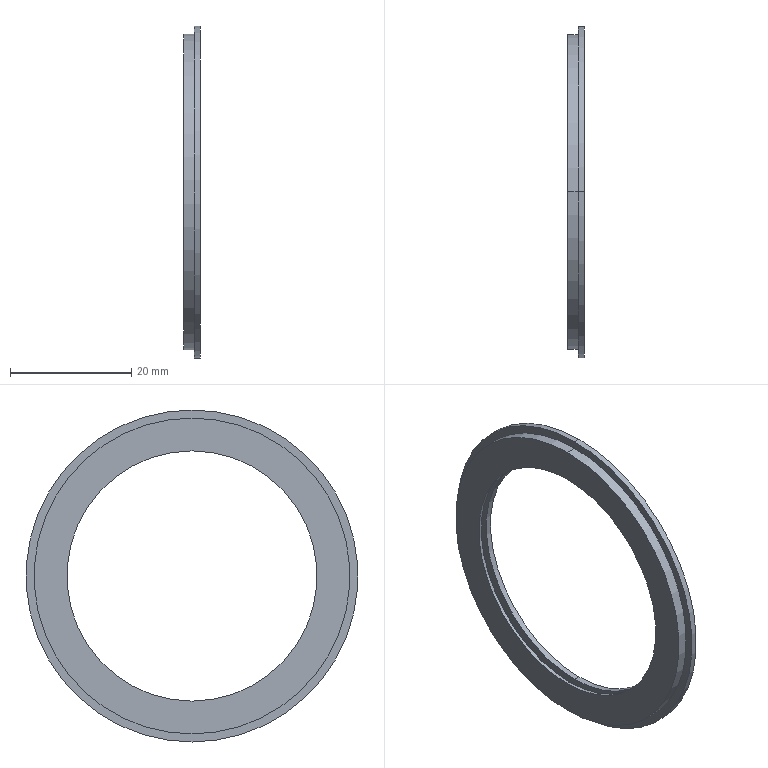Part | SolidWorks | features BaseBody 1 | 1 solid | 15 faces | box 2.7 x 54.668 x 54.668 mm | volume 1535 mm3 | cylinder 10 | plane 5 | commonest cylinder face diameters 41.2 x4 51 x2 52 x2 54.668 x2
STEP:
#1=CARTESIAN_POINT('',(-8.6,63.,15.566));
#2=VERTEX_POINT('',#1);
#3=CARTESIAN_POINT('',(-8.6,63.,70.234));
#4=VERTEX_POINT('',#3);
#5=CARTESIAN_POINT('',(-8.6,63.,42.9));
#6=DIRECTION('',(1.,0.,0.));
#7=DIRECTION('',(0.,0.,-1.));
#8=AXIS2_PLACEMENT_3D('',#5,#6,#7);
#9=CIRCLE('',#8,27.334);
#10=EDGE_CURVE('',#2,#4,#9,.T.);
#11=ORIENTED_EDGE('',*,*,#10,.T.);
#12=CARTESIAN_POINT('',(-7.6,63.,70.234));
#13=VERTEX_POINT('',#12);
#14=CARTESIAN_POINT('',(-8.1,63.,70.234));
#15=DIRECTION('',(1.,0.,0.));
#16=VECTOR('',#15,1000.);
#17=LINE('',#14,#16);
#18=EDGE_CURVE('',#4,#13,#17,.T.);
#19=ORIENTED_EDGE('',*,*,#18,.T.);
#20=CARTESIAN_POINT('',(-7.6,63.,15.566));
#21=VERTEX_POINT('',#20);
#22=CARTESIAN_POINT('',(-7.6,63.,42.9));
#23=DIRECTION('',(1.,0.,0.));
#24=DIRECTION('',(0.,0.,-1.));
#25=AXIS2_PLACEMENT_3D('',#22,#23,#24);
#26=CIRCLE('',#25,27.334);
#27=EDGE_CURVE('',#21,#13,#26,.T.);
#28=ORIENTED_EDGE('',*,*,#27,.F.);
#29=CARTESIAN_POINT('',(-8.1,63.,15.566));
#30=DIRECTION('',(1.,0.,0.));
#31=VECTOR('',#30,1000.);
#32=LINE('',#29,#31);
#33=EDGE_CURVE('',#2,#21,#32,.T.);
#34=ORIENTED_EDGE('',*,*,#33,.F.);
#35=EDGE_LOOP('',(#11,#19,#28,#34));
#36=FACE_OUTER_BOUND('',#35,.T.);
#37=CARTESIAN_POINT('',(-8.1,63.,42.9));
#38=DIRECTION('',(1.,0.,0.));
#39=DIRECTION('',(0.,0.,-1.));
#40=AXIS2_PLACEMENT_3D('',#37,#38,#39);
#41=CYLINDRICAL_SURFACE('',#40,27.334);
#42=ADVANCED_FACE('',(#36),#41,.T.);
#43=CARTESIAN_POINT('',(-8.6,63.,22.3));
#44=VERTEX_POINT('',#43);
#45=CARTESIAN_POINT('',(-8.6,63.,63.5));
#46=VERTEX_POINT('',#45);
#47=CARTESIAN_POINT('',(-8.6,63.,42.9));
#48=DIRECTION('',(-1.,0.,0.));
#49=DIRECTION('',(0.,0.,-1.));
#50=AXIS2_PLACEMENT_3D('',#47,#48,#49);
#51=CIRCLE('',#50,20.6);
#52=EDGE_CURVE('',#44,#46,#51,.T.);
#53=ORIENTED_EDGE('',*,*,#52,.T.);
#54=CARTESIAN_POINT('',(-7.6,63.,63.5));
#55=VERTEX_POINT('',#54);
#56=CARTESIAN_POINT('',(-8.6,63.,63.5));
#57=DIRECTION('',(1.,0.,0.));
#58=VECTOR('',#57,1000.);
#59=LINE('',#56,#58);
#60=EDGE_CURVE('',#46,#55,#59,.T.);
#61=ORIENTED_EDGE('',*,*,#60,.T.);
#62=CARTESIAN_POINT('',(-7.6,63.,22.3));
#63=VERTEX_POINT('',#62);
#64=CARTESIAN_POINT('',(-7.6,63.,42.9));
#65=DIRECTION('',(-1.,0.,0.));
#66=DIRECTION('',(0.,0.,-1.));
#67=AXIS2_PLACEMENT_3D('',#64,#65,#66);
#68=CIRCLE('',#67,20.6);
#69=EDGE_CURVE('',#63,#55,#68,.T.);
#70=ORIENTED_EDGE('',*,*,#69,.F.);
#71=CARTESIAN_POINT('',(-8.6,63.,22.3));
#72=DIRECTION('',(1.,0.,0.));
#73=VECTOR('',#72,1000.);
#74=LINE('',#71,#73);
#75=EDGE_CURVE('',#44,#63,#74,.T.);
#76=ORIENTED_EDGE('',*,*,#75,.F.);
#77=EDGE_LOOP('',(#53,#61,#70,#76));
#78=FACE_OUTER_BOUND('',#77,.T.);
#79=CARTESIAN_POINT('',(-8.6,63.,42.9));
#80=DIRECTION('',(1.,0.,0.));
#81=DIRECTION('',(0.,0.,-1.));
#82=AXIS2_PLACEMENT_3D('',#79,#80,#81);
#83=CYLINDRICAL_SURFACE('',#82,20.6);
#84=ADVANCED_FACE('',(#78),#83,.F.);
#85=CARTESIAN_POINT('',(-10.3,63.,16.9));
#86=VERTEX_POINT('',#85);
#87=CARTESIAN_POINT('',(-10.3,63.,68.9));
#88=VERTEX_POINT('',#87);
#89=CARTESIAN_POINT('',(-10.3,63.,42.9));
#90=DIRECTION('',(1.,0.,0.));
#91=DIRECTION('',(0.,0.,-1.));
#92=AXIS2_PLACEMENT_3D('',#89,#90,#91);
#93=CIRCLE('',#92,26.);
#94=EDGE_CURVE('',#86,#88,#93,.T.);
#95=ORIENTED_EDGE('',*,*,#94,.T.);
#96=CARTESIAN_POINT('',(-8.6,63.,68.9));
#97=VERTEX_POINT('',#96);
#98=CARTESIAN_POINT('',(-9.45,63.,68.9));
#99=DIRECTION('',(1.,0.,0.));
#100=VECTOR('',#99,1000.);
#101=LINE('',#98,#100);
#102=EDGE_CURVE('',#88,#97,#101,.T.);
#103=ORIENTED_EDGE('',*,*,#102,.T.);
#104=CARTESIAN_POINT('',(-8.6,63.,16.9));
#105=VERTEX_POINT('',#104);
#106=CARTESIAN_POINT('',(-8.6,63.,42.9));
#107=DIRECTION('',(1.,0.,0.));
#108=DIRECTION('',(0.,0.,-1.));
#109=AXIS2_PLACEMENT_3D('',#106,#107,#108);
#110=CIRCLE('',#109,26.);
#111=EDGE_CURVE('',#105,#97,#110,.T.);
#112=ORIENTED_EDGE('',*,*,#111,.F.);
#113=CARTESIAN_POINT('',(-9.45,63.,16.9));
#114=DIRECTION('',(1.,0.,0.));
#115=VECTOR('',#114,1000.);
#116=LINE('',#113,#115);
#117=EDGE_CURVE('',#86,#105,#116,.T.);
#118=ORIENTED_EDGE('',*,*,#117,.F.);
#119=EDGE_LOOP('',(#95,#103,#112,#118));
#120=FACE_OUTER_BOUND('',#119,.T.);
#121=CARTESIAN_POINT('',(-9.45,63.,42.9));
#122=DIRECTION('',(1.,0.,0.));
#123=DIRECTION('',(0.,0.,-1.));
#124=AXIS2_PLACEMENT_3D('',#121,#122,#123);
#125=CYLINDRICAL_SURFACE('',#124,26.);
#126=ADVANCED_FACE('',(#120),#125,.T.);
#127=CARTESIAN_POINT('',(-9.76,63.,17.4));
#128=VERTEX_POINT('',#127);
#129=CARTESIAN_POINT('',(-9.76,63.,68.4));
#130=VERTEX_POINT('',#129);
#131=CARTESIAN_POINT('',(-9.76,63.,42.9));
#132=DIRECTION('',(-1.,0.,0.));
#133=DIRECTION('',(0.,0.,-1.));
#134=AXIS2_PLACEMENT_3D('',#131,#132,#133);
#135=CIRCLE('',#134,25.5);
#136=EDGE_CURVE('',#128,#130,#135,.T.);
#137=ORIENTED_EDGE('',*,*,#136,.T.);
#138=CARTESIAN_POINT('',(-8.6,63.,68.4));
#139=VERTEX_POINT('',#138);
#140=CARTESIAN_POINT('',(-9.76,63.,68.4));
#141=DIRECTION('',(1.,0.,0.));
#142=VECTOR('',#141,1000.);
#143=LINE('',#140,#142);
#144=EDGE_CURVE('',#130,#139,#143,.T.);
#145=ORIENTED_EDGE('',*,*,#144,.T.);
#146=CARTESIAN_POINT('',(-8.6,63.,17.4));
#147=VERTEX_POINT('',#146);
#148=CARTESIAN_POINT('',(-8.6,63.,42.9));
#149=DIRECTION('',(-1.,0.,0.));
#150=DIRECTION('',(0.,0.,-1.));
#151=AXIS2_PLACEMENT_3D('',#148,#149,#150);
#152=CIRCLE('',#151,25.5);
#153=EDGE_CURVE('',#147,#139,#152,.T.);
#154=ORIENTED_EDGE('',*,*,#153,.F.);
#155=CARTESIAN_POINT('',(-9.76,63.,17.4));
#156=DIRECTION('',(1.,0.,0.));
#157=VECTOR('',#156,1000.);
#158=LINE('',#155,#157);
#159=EDGE_CURVE('',#128,#147,#158,.T.);
#160=ORIENTED_EDGE('',*,*,#159,.F.);
#161=EDGE_LOOP('',(#137,#145,#154,#160));
#162=FACE_OUTER_BOUND('',#161,.T.);
#163=CARTESIAN_POINT('',(-9.76,63.,42.9));
#164=DIRECTION('',(1.,0.,0.));
#165=DIRECTION('',(0.,0.,-1.));
#166=AXIS2_PLACEMENT_3D('',#163,#164,#165);
#167=CYLINDRICAL_SURFACE('',#166,25.5);
#168=ADVANCED_FACE('',(#162),#167,.F.);
#169=CARTESIAN_POINT('',(-10.3,63.,63.5));
#170=VERTEX_POINT('',#169);
#171=CARTESIAN_POINT('',(-10.3,63.,22.3));
#172=VERTEX_POINT('',#171);
#173=CARTESIAN_POINT('',(-10.3,63.,42.9));
#174=DIRECTION('',(1.,0.,0.));
#175=DIRECTION('',(0.,0.,-1.));
#176=AXIS2_PLACEMENT_3D('',#173,#174,#175);
#177=CIRCLE('',#176,20.6);
#178=EDGE_CURVE('',#170,#172,#177,.T.);
#179=ORIENTED_EDGE('',*,*,#178,.F.);
#180=CARTESIAN_POINT('',(-9.76,63.,63.5));
#181=VERTEX_POINT('',#180);
#182=CARTESIAN_POINT('',(-10.3,63.,63.5));
#183=DIRECTION('',(1.,0.,0.));
#184=VECTOR('',#183,1000.);
#185=LINE('',#182,#184);
#186=EDGE_CURVE('',#170,#181,#185,.T.);
#187=ORIENTED_EDGE('',*,*,#186,.T.);
#188=CARTESIAN_POINT('',(-9.76,63.,22.3));
#189=VERTEX_POINT('',#188);
#190=CARTESIAN_POINT('',(-9.76,63.,42.9));
#191=DIRECTION('',(-1.,0.,0.));
#192=DIRECTION('',(0.,0.,-1.));
#193=AXIS2_PLACEMENT_3D('',#190,#191,#192);
#194=CIRCLE('',#193,20.6);
#195=EDGE_CURVE('',#189,#181,#194,.T.);
#196=ORIENTED_EDGE('',*,*,#195,.F.);
#197=CARTESIAN_POINT('',(-10.3,63.,22.3));
#198=DIRECTION('',(1.,0.,0.));
#199=VECTOR('',#198,1000.);
#200=LINE('',#197,#199);
#201=EDGE_CURVE('',#172,#189,#200,.T.);
#202=ORIENTED_EDGE('',*,*,#201,.F.);
#203=EDGE_LOOP('',(#179,#187,#196,#202));
#204=FACE_OUTER_BOUND('',#203,.T.);
#205=CARTESIAN_POINT('',(-10.3,63.,42.9));
#206=DIRECTION('',(1.,0.,0.));
#207=DIRECTION('',(0.,0.,-1.));
#208=AXIS2_PLACEMENT_3D('',#205,#206,#207);
#209=CYLINDRICAL_SURFACE('',#208,20.6);
#210=ADVANCED_FACE('',(#204),#209,.F.);
#211=ORIENTED_EDGE('',*,*,#27,.T.);
#212=CARTESIAN_POINT('',(-7.6,63.,42.9));
#213=DIRECTION('',(1.,0.,0.));
#214=DIRECTION('',(0.,0.,-1.));
#215=AXIS2_PLACEMENT_3D('',#212,#213,#214);
#216=CIRCLE('',#215,27.334);
#217=EDGE_CURVE('',#13,#21,#216,.T.);
#218=ORIENTED_EDGE('',*,*,#217,.T.);
#219=EDGE_LOOP('',(#211,#218));
#220=FACE_OUTER_BOUND('',#219,.T.);
#221=ORIENTED_EDGE('',*,*,#69,.T.);
#222=CARTESIAN_POINT('',(-7.6,63.,42.9));
#223=DIRECTION('',(-1.,0.,0.));
#224=DIRECTION('',(0.,0.,-1.));
#225=AXIS2_PLACEMENT_3D('',#222,#223,#224);
#226=CIRCLE('',#225,20.6);
#227=EDGE_CURVE('',#55,#63,#226,.T.);
#228=ORIENTED_EDGE('',*,*,#227,.T.);
#229=EDGE_LOOP('',(#221,#228));
#230=FACE_BOUND('',#229,.T.);
#231=CARTESIAN_POINT('',(-7.6,63.,66.867));
#232=DIRECTION('',(1.,0.,0.));
#233=DIRECTION('',(0.,0.,-1.));
#234=AXIS2_PLACEMENT_3D('',#231,#232,#233);
#235=PLANE('',#234);
#236=ADVANCED_FACE('',(#220,#230),#235,.T.);
#237=ORIENTED_EDGE('',*,*,#18,.F.);
#238=CARTESIAN_POINT('',(-8.6,63.,42.9));
#239=DIRECTION('',(1.,0.,0.));
#240=DIRECTION('',(0.,0.,-1.));
#241=AXIS2_PLACEMENT_3D('',#238,#239,#240);
#242=CIRCLE('',#241,27.334);
#243=EDGE_CURVE('',#4,#2,#242,.T.);
#244=ORIENTED_EDGE('',*,*,#243,.T.);
#245=ORIENTED_EDGE('',*,*,#33,.T.);
#246=ORIENTED_EDGE('',*,*,#217,.F.);
#247=EDGE_LOOP('',(#237,#244,#245,#246));
#248=FACE_OUTER_BOUND('',#247,.T.);
#249=CARTESIAN_POINT('',(-8.1,63.,42.9));
#250=DIRECTION('',(1.,0.,0.));
#251=DIRECTION('',(0.,0.,-1.));
#252=AXIS2_PLACEMENT_3D('',#249,#250,#251);
#253=CYLINDRICAL_SURFACE('',#252,27.334);
#254=ADVANCED_FACE('',(#248),#253,.T.);
#255=ORIENTED_EDGE('',*,*,#60,.F.);
#256=CARTESIAN_POINT('',(-8.6,63.,42.9));
#257=DIRECTION('',(-1.,0.,0.));
#258=DIRECTION('',(0.,0.,-1.));
#259=AXIS2_PLACEMENT_3D('',#256,#257,#258);
#260=CIRCLE('',#259,20.6);
#261=EDGE_CURVE('',#46,#44,#260,.T.);
#262=ORIENTED_EDGE('',*,*,#261,.T.);
#263=ORIENTED_EDGE('',*,*,#75,.T.);
#264=ORIENTED_EDGE('',*,*,#227,.F.);
#265=EDGE_LOOP('',(#255,#262,#263,#264));
#266=FACE_OUTER_BOUND('',#265,.T.);
#267=CARTESIAN_POINT('',(-8.6,63.,42.9));
#268=DIRECTION('',(1.,0.,0.));
#269=DIRECTION('',(0.,0.,-1.));
#270=AXIS2_PLACEMENT_3D('',#267,#268,#269);
#271=CYLINDRICAL_SURFACE('',#270,20.6);
#272=ADVANCED_FACE('',(#266),#271,.F.);
#273=ORIENTED_EDGE('',*,*,#111,.T.);
#274=CARTESIAN_POINT('',(-8.6,63.,42.9));
#275=DIRECTION('',(1.,0.,0.));
#276=DIRECTION('',(0.,0.,-1.));
#277=AXIS2_PLACEMENT_3D('',#274,#275,#276);
#278=CIRCLE('',#277,26.);
#279=EDGE_CURVE('',#97,#105,#278,.T.);
#280=ORIENTED_EDGE('',*,*,#279,.T.);
#281=EDGE_LOOP('',(#273,#280));
#282=FACE_BOUND('',#281,.T.);
#283=ORIENTED_EDGE('',*,*,#10,.F.);
#284=ORIENTED_EDGE('',*,*,#243,.F.);
#285=EDGE_LOOP('',(#283,#284));
#286=FACE_OUTER_BOUND('',#285,.T.);
#287=CARTESIAN_POINT('',(-8.6,63.,69.567));
#288=DIRECTION('',(-1.,0.,0.));
#289=DIRECTION('',(0.,0.,1.));
#290=AXIS2_PLACEMENT_3D('',#287,#288,#289);
#291=PLANE('',#290);
#292=ADVANCED_FACE('',(#282,#286),#291,.T.);
#293=ORIENTED_EDGE('',*,*,#52,.F.);
#294=ORIENTED_EDGE('',*,*,#261,.F.);
#295=EDGE_LOOP('',(#293,#294));
#296=FACE_BOUND('',#295,.T.);
#297=ORIENTED_EDGE('',*,*,#153,.T.);
#298=CARTESIAN_POINT('',(-8.6,63.,42.9));
#299=DIRECTION('',(-1.,0.,0.));
#300=DIRECTION('',(0.,0.,-1.));
#301=AXIS2_PLACEMENT_3D('',#298,#299,#300);
#302=CIRCLE('',#301,25.5);
#303=EDGE_CURVE('',#139,#147,#302,.T.);
#304=ORIENTED_EDGE('',*,*,#303,.T.);
#305=EDGE_LOOP('',(#297,#304));
#306=FACE_OUTER_BOUND('',#305,.T.);
#307=CARTESIAN_POINT('',(-8.6,63.,65.95));
#308=DIRECTION('',(-1.,0.,0.));
#309=DIRECTION('',(0.,0.,1.));
#310=AXIS2_PLACEMENT_3D('',#307,#308,#309);
#311=PLANE('',#310);
#312=ADVANCED_FACE('',(#296,#306),#311,.T.);
#313=ORIENTED_EDGE('',*,*,#102,.F.);
#314=CARTESIAN_POINT('',(-10.3,63.,42.9));
#315=DIRECTION('',(1.,0.,0.));
#316=DIRECTION('',(0.,0.,-1.));
#317=AXIS2_PLACEMENT_3D('',#314,#315,#316);
#318=CIRCLE('',#317,26.);
#319=EDGE_CURVE('',#88,#86,#318,.T.);
#320=ORIENTED_EDGE('',*,*,#319,.T.);
#321=ORIENTED_EDGE('',*,*,#117,.T.);
#322=ORIENTED_EDGE('',*,*,#279,.F.);
#323=EDGE_LOOP('',(#313,#320,#321,#322));
#324=FACE_OUTER_BOUND('',#323,.T.);
#325=CARTESIAN_POINT('',(-9.45,63.,42.9));
#326=DIRECTION('',(1.,0.,0.));
#327=DIRECTION('',(0.,0.,-1.));
#328=AXIS2_PLACEMENT_3D('',#325,#326,#327);
#329=CYLINDRICAL_SURFACE('',#328,26.);
#330=ADVANCED_FACE('',(#324),#329,.T.);
#331=ORIENTED_EDGE('',*,*,#144,.F.);
#332=CARTESIAN_POINT('',(-9.76,63.,42.9));
#333=DIRECTION('',(-1.,0.,0.));
#334=DIRECTION('',(0.,0.,-1.));
#335=AXIS2_PLACEMENT_3D('',#332,#333,#334);
#336=CIRCLE('',#335,25.5);
#337=EDGE_CURVE('',#130,#128,#336,.T.);
#338=ORIENTED_EDGE('',*,*,#337,.T.);
#339=ORIENTED_EDGE('',*,*,#159,.T.);
#340=ORIENTED_EDGE('',*,*,#303,.F.);
#341=EDGE_LOOP('',(#331,#338,#339,#340));
#342=FACE_OUTER_BOUND('',#341,.T.);
#343=CARTESIAN_POINT('',(-9.76,63.,42.9));
#344=DIRECTION('',(1.,0.,0.));
#345=DIRECTION('',(0.,0.,-1.));
#346=AXIS2_PLACEMENT_3D('',#343,#344,#345);
#347=CYLINDRICAL_SURFACE('',#346,25.5);
#348=ADVANCED_FACE('',(#342),#347,.F.);
#349=CARTESIAN_POINT('',(-10.3,63.,42.9));
#350=DIRECTION('',(1.,0.,0.));
#351=DIRECTION('',(0.,0.,-1.));
#352=AXIS2_PLACEMENT_3D('',#349,#350,#351);
#353=CIRCLE('',#352,20.6);
#354=EDGE_CURVE('',#172,#170,#353,.T.);
#355=ORIENTED_EDGE('',*,*,#354,.T.);
#356=ORIENTED_EDGE('',*,*,#178,.T.);
#357=EDGE_LOOP('',(#355,#356));
#358=FACE_BOUND('',#357,.T.);
#359=ORIENTED_EDGE('',*,*,#94,.F.);
#360=ORIENTED_EDGE('',*,*,#319,.F.);
#361=EDGE_LOOP('',(#359,#360));
#362=FACE_OUTER_BOUND('',#361,.T.);
#363=CARTESIAN_POINT('',(-10.3,63.,66.2));
#364=DIRECTION('',(-1.,0.,0.));
#365=DIRECTION('',(0.,0.,1.));
#366=AXIS2_PLACEMENT_3D('',#363,#364,#365);
#367=PLANE('',#366);
#368=ADVANCED_FACE('',(#358,#362),#367,.T.);
#369=ORIENTED_EDGE('',*,*,#136,.F.);
#370=ORIENTED_EDGE('',*,*,#337,.F.);
#371=EDGE_LOOP('',(#369,#370));
#372=FACE_OUTER_BOUND('',#371,.T.);
#373=ORIENTED_EDGE('',*,*,#195,.T.);
#374=CARTESIAN_POINT('',(-9.76,63.,42.9));
#375=DIRECTION('',(-1.,0.,0.));
#376=DIRECTION('',(0.,0.,-1.));
#377=AXIS2_PLACEMENT_3D('',#374,#375,#376);
#378=CIRCLE('',#377,20.6);
#379=EDGE_CURVE('',#181,#189,#378,.T.);
#380=ORIENTED_EDGE('',*,*,#379,.T.);
#381=EDGE_LOOP('',(#373,#380));
#382=FACE_BOUND('',#381,.T.);
#383=CARTESIAN_POINT('',(-9.76,63.,65.95));
#384=DIRECTION('',(1.,0.,0.));
#385=DIRECTION('',(0.,0.,-1.));
#386=AXIS2_PLACEMENT_3D('',#383,#384,#385);
#387=PLANE('',#386);
#388=ADVANCED_FACE('',(#372,#382),#387,.T.);
#389=ORIENTED_EDGE('',*,*,#186,.F.);
#390=ORIENTED_EDGE('',*,*,#354,.F.);
#391=ORIENTED_EDGE('',*,*,#201,.T.);
#392=ORIENTED_EDGE('',*,*,#379,.F.);
#393=EDGE_LOOP('',(#389,#390,#391,#392));
#394=FACE_OUTER_BOUND('',#393,.T.);
#395=CARTESIAN_POINT('',(-10.3,63.,42.9));
#396=DIRECTION('',(1.,0.,0.));
#397=DIRECTION('',(0.,0.,-1.));
#398=AXIS2_PLACEMENT_3D('',#395,#396,#397);
#399=CYLINDRICAL_SURFACE('',#398,20.6);
#400=ADVANCED_FACE('',(#394),#399,.F.);
#401=CLOSED_SHELL('',(#42,#84,#126,#168,#210,#236,#254,#272,#292,#312,#330,#348,#368,#388,#400));
#402=MANIFOLD_SOLID_BREP('',#401);
#403=CARTESIAN_POINT('',(0.,0.,0.));
#404=DIRECTION('',(0.,0.,1.));
#405=DIRECTION('',(1.,0.,0.));
#406=AXIS2_PLACEMENT_3D('',#403,#404,#405);
#407=(LENGTH_UNIT()NAMED_UNIT(*)SI_UNIT(.MILLI.,.METRE.));
#408=UNCERTAINTY_MEASURE_WITH_UNIT(LENGTH_MEASURE(0.00001),#407,'','');
#409=(NAMED_UNIT(*)PLANE_ANGLE_UNIT()SI_UNIT($,.RADIAN.));
#410=(NAMED_UNIT(*)SI_UNIT($,.STERADIAN.)SOLID_ANGLE_UNIT());
#411=(GEOMETRIC_REPRESENTATION_CONTEXT(3)GLOBAL_UNCERTAINTY_ASSIGNED_CONTEXT((#408))GLOBAL_UNIT_ASSIGNED_CONTEXT((#407,#409,#410))REPRESENTATION_CONTEXT('',''));
#412=ADVANCED_BREP_SHAPE_REPRESENTATION('',(#402,#406),#411);